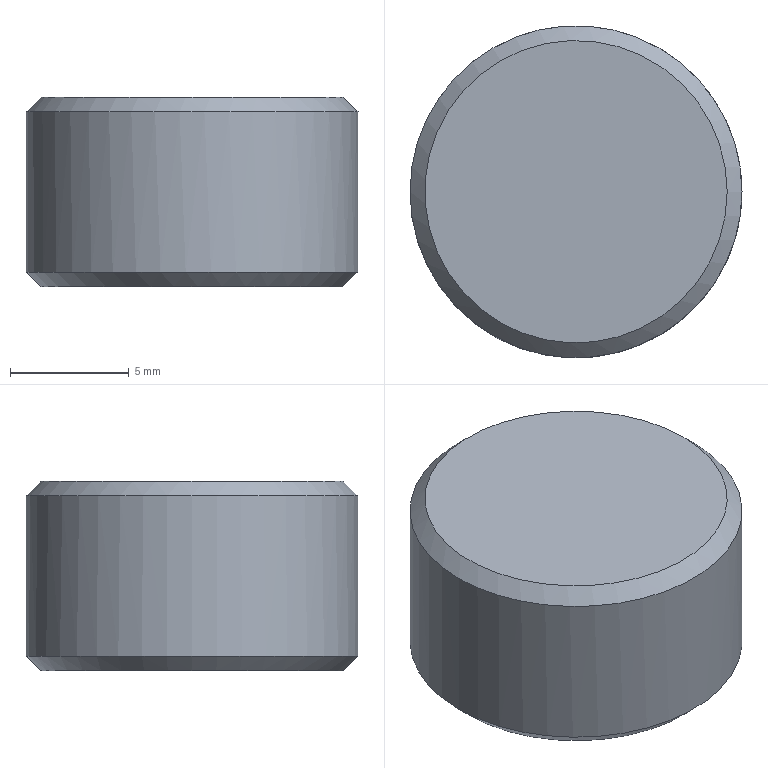Part | NX | features PG_666 2 | 1 solid | 5 faces | box 14 x 14 x 8 mm | volume 1215 mm3 | plane 2 | cone 2 | cylinder 1 | commonest cylinder face diameters 14 x1
STEP:
#1=CARTESIAN_POINT('',(3799.713,-824.144,742.716));
#2=VERTEX_POINT('',#1);
#3=CARTESIAN_POINT('',(3806.088,-824.144,742.716));
#4=DIRECTION('',(0.,0.,1.));
#5=DIRECTION('',(-1.,0.,0.));
#6=AXIS2_PLACEMENT_3D('',#3,#4,#5);
#7=CIRCLE('',#6,6.375);
#8=EDGE_CURVE('',#2,#2,#7,.T.);
#9=ORIENTED_EDGE('',*,*,#8,.F.);
#10=EDGE_LOOP('',(#9));
#11=FACE_BOUND('',#10,.T.);
#12=CARTESIAN_POINT('',(3806.088,-824.144,742.716));
#13=DIRECTION('',(0.,0.,-1.));
#14=DIRECTION('',(-1.,0.,0.));
#15=AXIS2_PLACEMENT_3D('',#12,#13,#14);
#16=PLANE('',#15);
#17=ADVANCED_FACE('',(#11),#16,.T.);
#18=CARTESIAN_POINT('',(3812.463,-824.144,750.716));
#19=VERTEX_POINT('',#18);
#20=CARTESIAN_POINT('',(3806.088,-824.144,750.716));
#21=DIRECTION('',(0.,0.,-1.));
#22=DIRECTION('',(1.,0.,0.));
#23=AXIS2_PLACEMENT_3D('',#20,#21,#22);
#24=CIRCLE('',#23,6.375);
#25=EDGE_CURVE('',#19,#19,#24,.T.);
#26=ORIENTED_EDGE('',*,*,#25,.F.);
#27=EDGE_LOOP('',(#26));
#28=FACE_BOUND('',#27,.T.);
#29=CARTESIAN_POINT('',(3806.088,-824.144,750.716));
#30=DIRECTION('',(0.,0.,1.));
#31=DIRECTION('',(1.,0.,0.));
#32=AXIS2_PLACEMENT_3D('',#29,#30,#31);
#33=PLANE('',#32);
#34=ADVANCED_FACE('',(#28),#33,.T.);
#35=CARTESIAN_POINT('',(3813.088,-824.144,750.091));
#36=VERTEX_POINT('',#35);
#37=CARTESIAN_POINT('',(3806.088,-824.144,750.091));
#38=DIRECTION('',(0.,0.,-1.));
#39=DIRECTION('',(1.,0.,0.));
#40=AXIS2_PLACEMENT_3D('',#37,#38,#39);
#41=CIRCLE('',#40,7.);
#42=EDGE_CURVE('',#36,#36,#41,.F.);
#43=ORIENTED_EDGE('',*,*,#42,.F.);
#44=EDGE_LOOP('',(#43));
#45=FACE_BOUND('',#44,.T.);
#46=CARTESIAN_POINT('',(3799.088,-824.144,743.341));
#47=VERTEX_POINT('',#46);
#48=CARTESIAN_POINT('',(3806.088,-824.144,743.341));
#49=DIRECTION('',(0.,0.,1.));
#50=DIRECTION('',(-1.,0.,0.));
#51=AXIS2_PLACEMENT_3D('',#48,#49,#50);
#52=CIRCLE('',#51,7.);
#53=EDGE_CURVE('',#47,#47,#52,.F.);
#54=ORIENTED_EDGE('',*,*,#53,.F.);
#55=EDGE_LOOP('',(#54));
#56=FACE_BOUND('',#55,.T.);
#57=CARTESIAN_POINT('',(3806.088,-824.144,811.716));
#58=DIRECTION('',(0.,0.,-1.));
#59=DIRECTION('',(-1.,0.,0.));
#60=AXIS2_PLACEMENT_3D('',#57,#58,#59);
#61=CYLINDRICAL_SURFACE('',#60,7.);
#62=ADVANCED_FACE('',(#45,#56),#61,.T.);
#63=ORIENTED_EDGE('',*,*,#25,.T.);
#64=EDGE_LOOP('',(#63));
#65=FACE_BOUND('',#64,.T.);
#66=ORIENTED_EDGE('',*,*,#42,.T.);
#67=EDGE_LOOP('',(#66));
#68=FACE_BOUND('',#67,.T.);
#69=CARTESIAN_POINT('',(3806.088,-824.144,750.091));
#70=DIRECTION('',(0.,0.,-1.));
#71=DIRECTION('',(-1.,0.,0.));
#72=AXIS2_PLACEMENT_3D('',#69,#70,#71);
#73=CONICAL_SURFACE('',#72,7.,0.7854);
#74=ADVANCED_FACE('',(#65,#68),#73,.T.);
#75=ORIENTED_EDGE('',*,*,#8,.T.);
#76=EDGE_LOOP('',(#75));
#77=FACE_BOUND('',#76,.T.);
#78=ORIENTED_EDGE('',*,*,#53,.T.);
#79=EDGE_LOOP('',(#78));
#80=FACE_BOUND('',#79,.T.);
#81=CARTESIAN_POINT('',(3806.088,-824.144,743.341));
#82=DIRECTION('',(0.,0.,1.));
#83=DIRECTION('',(1.,0.,0.));
#84=AXIS2_PLACEMENT_3D('',#81,#82,#83);
#85=CONICAL_SURFACE('',#84,7.,0.7854);
#86=ADVANCED_FACE('',(#77,#80),#85,.T.);
#87=CLOSED_SHELL('',(#17,#34,#62,#74,#86));
#88=MANIFOLD_SOLID_BREP('',#87);
#89=(LENGTH_UNIT()NAMED_UNIT(*)SI_UNIT(.MILLI.,.METRE.));
#90=UNCERTAINTY_MEASURE_WITH_UNIT(LENGTH_MEASURE(0.00001),#89,'','');
#91=(NAMED_UNIT(*)PLANE_ANGLE_UNIT()SI_UNIT($,.RADIAN.));
#92=(NAMED_UNIT(*)SI_UNIT($,.STERADIAN.)SOLID_ANGLE_UNIT());
#93=(GEOMETRIC_REPRESENTATION_CONTEXT(3)GLOBAL_UNCERTAINTY_ASSIGNED_CONTEXT((#90))GLOBAL_UNIT_ASSIGNED_CONTEXT((#89,#91,#92))REPRESENTATION_CONTEXT('',''));
#94=ADVANCED_BREP_SHAPE_REPRESENTATION('',(#88),#93);